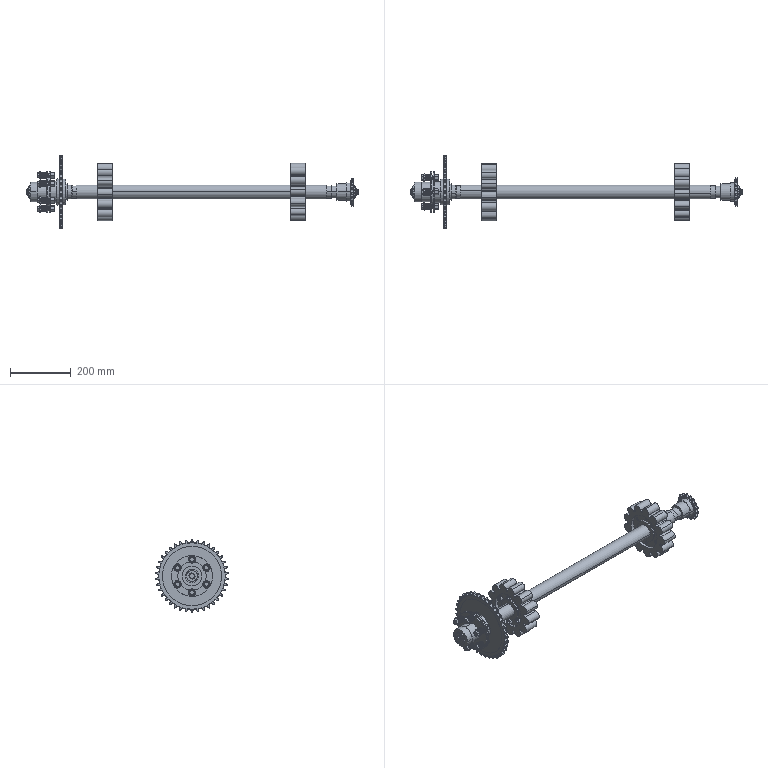Part | SolidWorks | features ReferencePattern 30, CompositeCurve 4, LocalCirPattern 3, AEMSimFeature 1 | 65 solids | 4154 faces | volume 4579518 mm3 | cone 1658 | cylinder 1630 | plane 596 | torus 222 | spline 48 | commonest cylinder face diameters 10 x616 12 x238 17.009 x80 31.126 x78 8.5 x52 28.613 x52